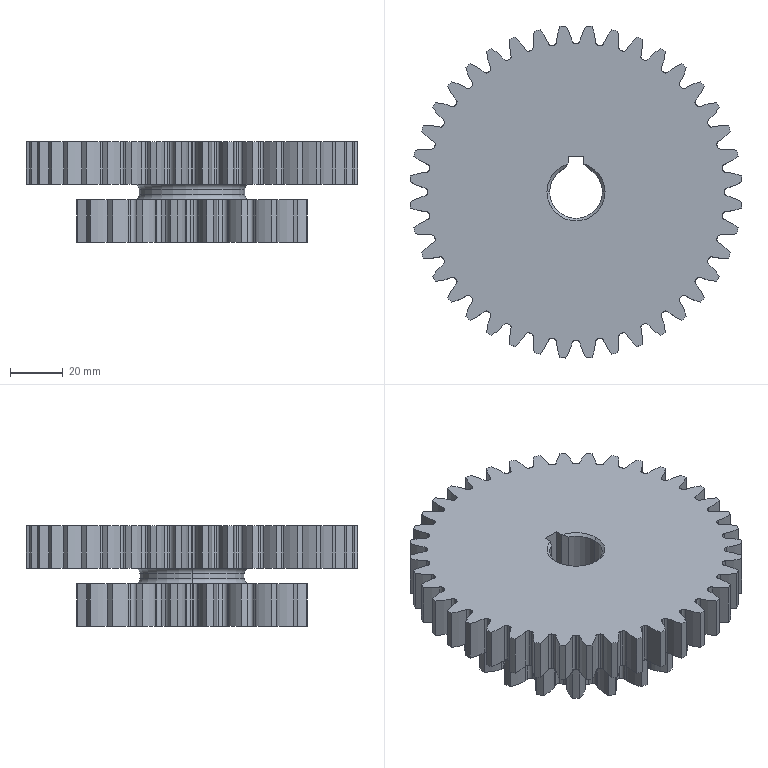Part | SolidWorks | features BaseBody 1 | 1 solid | 454 faces | box 125.77 x 125.77 x 38 mm | volume 253321 mm3 | cylinder 275 | spline 120 | plane 49 | cone 6 | torus 4 | commonest cylinder face diameters 2.28 x98 3.04 x50 112.5 x41 126 x40 70 x21 88 x20